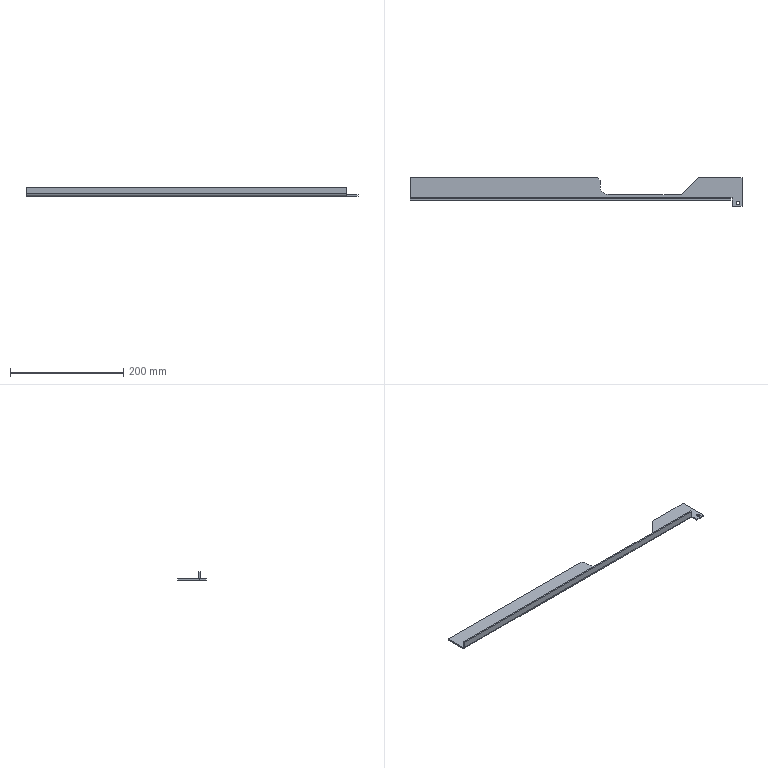Part | STEP file | 1 solid | 23 faces | box 587 x 51 x 15 mm | volume 63282 mm3 | plane 17 | cylinder 6 | commonest cylinder face diameters 6 x2 3 x1 8 x1 20 x1 30 x1